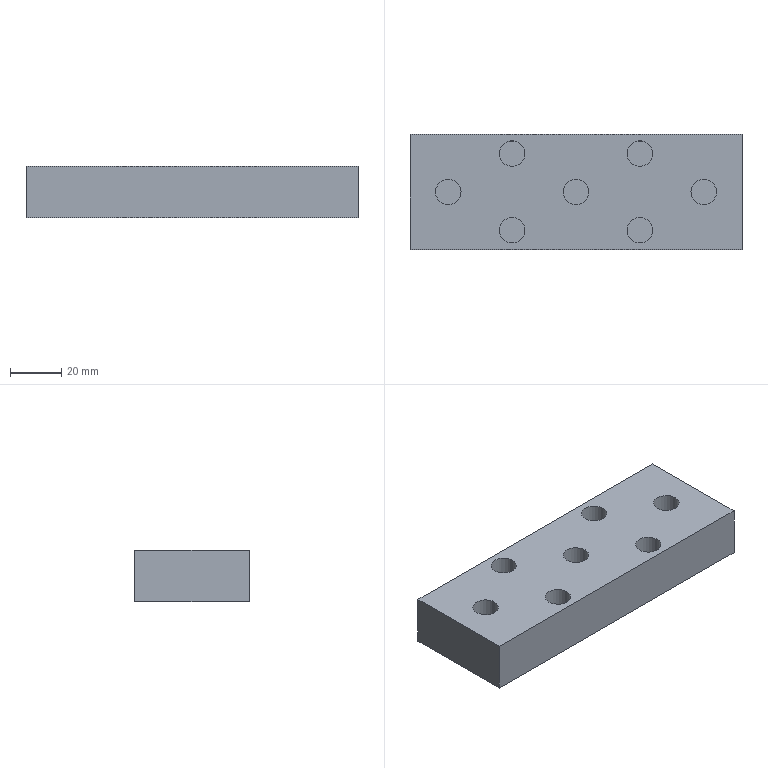NC program | NX | posted with a generic post | part box 130 x 45 x 20 mm
Lines 1 to 287 of 3690:
N10 G17 G21 G94 G90
(PLANAR_MILL , TOOL : D63R0.8)
N12 T01 M6
N14 G54
N16 G17 G0 G90 X128. Y1. S3500 M3
N18 G43 Z30. H1
N20 Z3.
N22 G94 G1 Z0. F800.
N24 X65.
N26 X-65.
N28 X-128.
N30 Z3.
N32 G0 Z30.
N34 M5
(ADAPTIVE_MILLING , TOOL : D10开粗)
N36 T07 M6
N38 G54
N40 G17 G0 G90 X-78.055 Y-23.628 S5500 M3
N42 G43 Z30. H7
N44 Z-17.
N46 G94 G1 X-77.905 Y-23.625 Z-17.937 F2500.
N48 X-77.755 Y-23.623 Z-18.308
N50 X-77.605 Y-23.62 Z-18.58
N52 X-77.455 Y-23.617 Z-18.8
N54 X-77.305 Y-23.614 Z-18.984
N56 X-77.155 Y-23.612 Z-19.142
N58 X-77.005 Y-23.609 Z-19.28
N60 X-76.855 Y-23.606 Z-19.4
N62 X-76.705 Y-23.604 Z-19.505
N64 X-76.555 Y-23.601 Z-19.598
N66 X-76.405 Y-23.598 Z-19.679
N68 X-76.255 Y-23.596 Z-19.75
N70 X-76.105 Y-23.593 Z-19.81
N72 X-75.955 Y-23.59 Z-19.862
N74 X-75.805 Y-23.588 Z-19.905
N76 X-75.655 Y-23.585 Z-19.939
N78 X-75.505 Y-23.582 Z-19.966
N80 X-75.355 Y-23.58 Z-19.985
N82 X-75.205 Y-23.577 Z-19.996
N84 X-75.055 Y-23.574 Z-20.
N86 X-73.461 Y-23.546
N88 G3 X-72.537 Y-22.899 R1.011
N90 X-72.311 Y-22.012 R4.081
N92 X-72.087 Y-19.387 R22.214
N94 X-72.006 Y-13.376 R176.752
N96 G1 X-71.999 Y21.926
N98 X-71.986 Y23.238
N100 G2 X-70.794 Y26.144 R5.335
N102 X-68.247 Y28.119 R7.268
N104 X-65.211 Y29.054 R11.643
N106 X-61.605 Y29.404 R27.82
N108 X-55.731 Y29.494 R158.029
N110 G1 X64.423 Y29.499
N112 X65.735 Y29.486
N114 G2 X68.641 Y28.295 R5.335
N116 X70.617 Y25.748 R7.269
N118 X71.553 Y22.712 R11.647
N120 X71.904 Y19.107 R27.781
N122 X71.994 Y13.233 R157.657
N124 G1 X72. Y-21.86
N126 X71.987 Y-23.235
N128 G2 X70.796 Y-26.141 R5.334
N130 X68.25 Y-28.116 R7.264
N132 X65.211 Y-29.051 R11.685
N134 X61.668 Y-29.399 R27.556
N136 X55.795 Y-29.492 R153.539
N138 G1 X-64.237 Y-29.499
N140 X-65.737 Y-29.485
N142 G2 X-68.642 Y-28.295 R5.336
N144 X-70.46 Y-25.898 R6.534
N146 X-71.246 Y-23.143 R10.299
N148 X-71.485 Y-19.966 R25.361
N150 G1 X-71.511 Y-16.966
N152 X-71.508 Y20.191
N154 X-71.493 Y21.124
N156 G2 X-69.391 Y25.736 R6.967
N158 X-66.353 Y27.691 R9.166
N160 X-62.911 Y28.584 R14.965
N162 X-58.863 Y28.912 R36.984
N164 X-51.864 Y28.996 R226.939
N166 G1 X61.8 Y29.
N168 X63.674 Y28.985
N170 G2 X68.272 Y26.852 R6.98
N172 X70.212 Y23.798 R9.229
N174 X71.082 Y20.416 R15.042
N176 X71.416 Y16.244 R37.366
N178 X71.496 Y9.12 R241.015
N180 G1 X71.5 Y-19.36
N182 X71.486 Y-21.173
N184 G2 X69.441 Y-25.683 R6.948
N186 X66.467 Y-27.642 R9.044
N188 X63.033 Y-28.563 R14.686
N190 X58.988 Y-28.905 R35.495
N192 X52.239 Y-28.993 R208.132
N194 G1 X-62.237 Y-28.998
N196 X-63.799 Y-28.977
N198 G2 X-68.052 Y-26.942 R6.612
N200 X-69.639 Y-24.587 R8.401
N202 X-70.01 Y-23.694 R5.86
N204 X-70.726 Y-20.401 R15.34
N206 X-70.964 Y-16.285 R43.956
N208 X-71.01 Y-7.535 R498.765
N210 G1 Y16.09
N212 X-71.004 Y19.278
N214 G2 X-70.114 Y22.888 R8.361
N216 G3 X-70.002 Y23.496 R2.149
N218 G2 X-69.24 Y25.334 R5.933
N220 X-67.832 Y26.741 R5.933
N222 G1 X-66.95 Y27.212
N224 X-65.933 Y27.516
N226 G2 X-58.616 Y28.374 R44.657
N228 X-51.617 Y28.491 R189.581
N230 G1 X-44.617 Y28.499
N232 X61.633 Y28.497
N234 G2 X64.861 Y27.853 R8.581
N236 G3 X65.996 Y27.502 R2.55
N238 G2 X67.835 Y26.74 R5.933
N240 X69.241 Y25.332 R5.933
N242 G1 X69.712 Y24.45
N244 X70.016 Y23.433
N246 G2 X70.874 Y16.113 R44.791
N248 X70.991 Y9.114 R189.425
N250 G1 X71. Y2.114
N252 X70.997 Y-19.136
N254 G2 X70.328 Y-22.421 R8.526
N256 G3 X70.002 Y-23.496 R2.362
N258 G2 X69.24 Y-25.335 R5.933
N260 X67.832 Y-26.741 R5.933
N262 G1 X66.95 Y-27.212
N264 X65.933 Y-27.516
N266 G2 X58.609 Y-28.373 R44.955
N268 X51.611 Y-28.489 R189.681
N270 G1 X-60.299 Y-28.498
N272 X-62.174 Y-28.468
N274 G2 X-65.223 Y-27.62 R7.754
N276 G3 X-65.997 Y-27.502 R3.16
N278 G2 X-67.835 Y-26.739 R5.933
N280 X-69.241 Y-25.332 R5.933
N282 X-70.002 Y-23.493 R5.933
N284 X-70.498 Y-11.529 R124.107
N286 G1 X-70.51 Y-3.904
N288 X-70.506 Y19.096
N290 X-70.1 Y20.983
N292 G2 X-70.032 Y23.185 R15.461
N294 G3 X-71.266 Y24.254 R1.
N296 X-71.91 Y23.763 Z-19.958 R1.058
N298 G1 X-72.554 Y22.81 Z-19.9
N300 X-73.241 Y21.791 F15000.
N302 G3 X-73.412 Y21.234 R1.01
N304 G1 X-73.48 Y-20.549
N306 G3 X-73.296 Y-21.128 R1.009
N308 G1 X-72.588 Y-22.129
N310 X-71.873 Y-23.131 Z-19.962 F2500.
N312 G3 X-71.234 Y-23.491 Z-20. R1.001
N314 X-70.1 Y-22.5 R1.
N316 G1 Y22.501
N318 G2 X-69.711 Y24.453 R5.936
N320 X-68.605 Y26.107 R5.933
N322 X-66.95 Y27.212 R5.933
N324 X-65. Y27.6 R5.938
N326 G3 X-60.266 Y27.784 R66.229
N328 G2 X-47.769 Y27.996 R256.874
N330 G1 X-43.144 Y27.999
N332 X60.262 Y27.994
N334 G2 X63.174 Y27.6 R15.263
N336 G1 X65.001
N338 X65.685 Y27.532
N340 G3 X66.755 Y28.763 R1.
N342 X66.265 Y29.409 Z-19.958 R1.057
N344 G1 X65.313 Y30.053 Z-19.9
N346 X64.299 Y30.74 F15000.
N348 G3 X63.734 Y30.912 R1.01
N350 G1 X-61.177 Y30.36
N352 X-61.309 Y30.348
N354 X-61.438 Y30.324
N356 X-62.319 Y30.082
N358 X-64.23 Y29.556 Z-20. F2500.
N360 G3 X-63.937 Y27.6 R1.
N362 G1 X65.001
N364 G2 X66.953 Y27.211 R5.936
N366 X68.607 Y26.105 R5.933
N368 X69.712 Y24.45 R5.933
N370 X70.1 Y22.499 R5.938
N372 G3 X70.283 Y17.766 R66.243
N374 G2 X70.496 Y5.269 R256.704
N376 G1 X70.499 Y0.644
N378 X70.495 Y-18.637
N380 G2 X70.1 Y-20.799 R24.154
N382 X70.032 Y-23.185 R17.227
N384 G3 X71.258 Y-24.256 R1.
N386 X71.908 Y-23.767 Z-19.958 R1.057
N388 G1 X72.553 Y-22.819 Z-19.9
N390 X73.239 Y-21.81 F15000.
N392 G3 X73.412 Y-21.234 R1.009
N394 G1 X72.86 Y18.677
N396 X72.847 Y18.803
N398 X72.824 Y18.927
N400 X72.582 Y19.812
N402 X72.058 Y21.724 Z-20. F2500.
N404 G3 X70.1 Y21.437 R1.
N406 G1 Y-22.501
N408 G2 X69.711 Y-24.453 R5.936
N410 X68.605 Y-26.107 R5.933
N412 X66.95 Y-27.212 R5.933
N414 X64.999 Y-27.6 R5.938
N416 G3 X59.826 Y-27.804 R80.416
N418 G2 X46.828 Y-27.996 R290.508
N420 G1 X-59.951 Y-27.998
N422 G2 X-63.044 Y-27.6 R14.936
N424 G1 X-65.001
N426 X-65.499 Y-27.551
N428 G3 X-66.572 Y-28.77 R1.
N430 X-66.079 Y-29.427 Z-19.957 R1.056
N432 G1 X-65.137 Y-30.065 Z-19.9
N434 X-64.112 Y-30.759 F15000.
N436 G3 X-63.547 Y-30.931 R1.01
N438 G1 X61.177 Y-30.36
N440 X61.308 Y-30.348
N442 X61.438 Y-30.324
N444 X62.318 Y-30.082
N446 X64.229 Y-29.556 Z-20. F2500.
N448 G3 X63.937 Y-27.6 R1.
N450 G1 X-63.063
N452 G3 X-64.072 Y-28.554 R1.01
N454 G1 X-64.157 Y-30.078
N456 X-64.165 Y-30.228 Z-19.996
N458 X-64.174 Y-30.377 Z-19.985
N460 X-64.182 Y-30.527 Z-19.966
N462 X-64.19 Y-30.677 Z-19.939
N464 X-64.199 Y-30.827 Z-19.905
N466 X-64.207 Y-30.976 Z-19.862
N468 X-64.215 Y-31.126 Z-19.81
N470 X-64.224 Y-31.276 Z-19.75
N472 X-64.232 Y-31.426 Z-19.679
N474 X-64.241 Y-31.575 Z-19.598
N476 X-64.249 Y-31.725 Z-19.505
N478 X-64.257 Y-31.875 Z-19.4
N480 X-64.266 Y-32.025 Z-19.28
N482 X-64.274 Y-32.175 Z-19.142
N484 X-64.282 Y-32.324 Z-18.984
N486 X-64.291 Y-32.474 Z-18.8
N488 X-64.299 Y-32.624 Z-18.58
N490 X-64.307 Y-32.774 Z-18.308
N492 X-64.316 Y-32.923 Z-17.937
N494 X-64.324 Y-33.073 Z-17.
N496 G0 Z30.
N498 M5
(DRILLING , TOOL : D10点钻)
N500 T02 M6
N502 G54
N504 G17 G0 G90 X-50. Y0. S2000 M3
N506 G43 Z30. H2
N508 G94 G81 G98 Z-1.5 F200. R3.
N510 X-25. Y15.
N512 Y-15.
N514 X0. Y0.
N516 X25. Y15.
N518 Y-15.
N520 X50. Y0.
N522 G80
N524 G0 X50. Y0. Z30.
N526 M5
(DRILLING_COPY , TOOL : Z6.5)
N528 T04 M6
N530 G54
N532 G17 G0 G90 X-50. Y0. S3000 M3
N534 G43 Z30. H4
N536 G94 G81 G98 Z-10. F200. R3.
N538 X-25. Y15.
N540 Y-15.
N542 X0. Y0.
N544 X25. Y15.
N546 Y-15.
N548 X50. Y0.
N550 G80
N552 G0 X50. Y0. Z30.
N554 M5